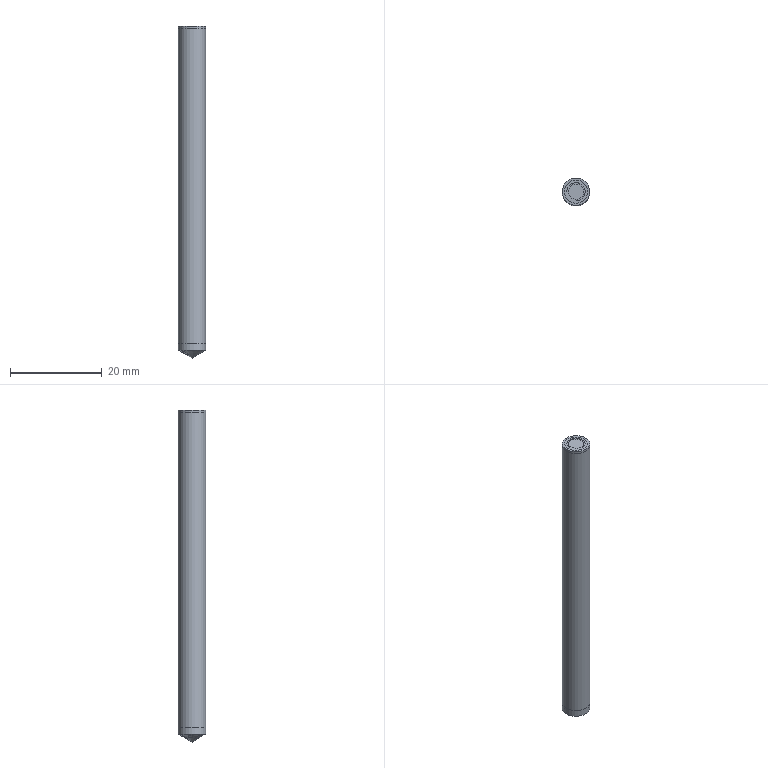Part | STEP file | EE030607000 | 2 solids | 45 faces | box 6 x 6 x 72.232 mm | volume 3898 mm3 | plane 15 | other 13 | cone 11 | cylinder 5 | torus 1 | commonest cylinder face diameters 6 x2 3.333 x1 3.987 x1 4 x1